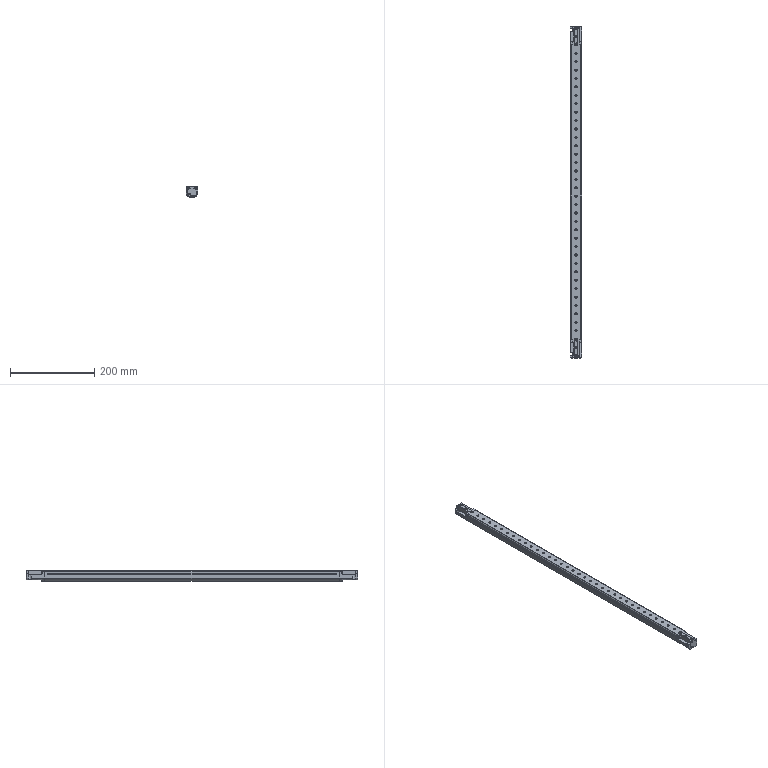Part | STEP file | Guide wheel mechanism revised.sldasm-Part-315 | 1 solid | 362 faces | box 28 x 790 x 26.2 mm | volume 498619 mm3 | cylinder 191 | plane 159 | spline 12 | commonest cylinder face diameters 5 x84 0.5 x12 3 x12 4.5 x12 4.9 x12 32 x11